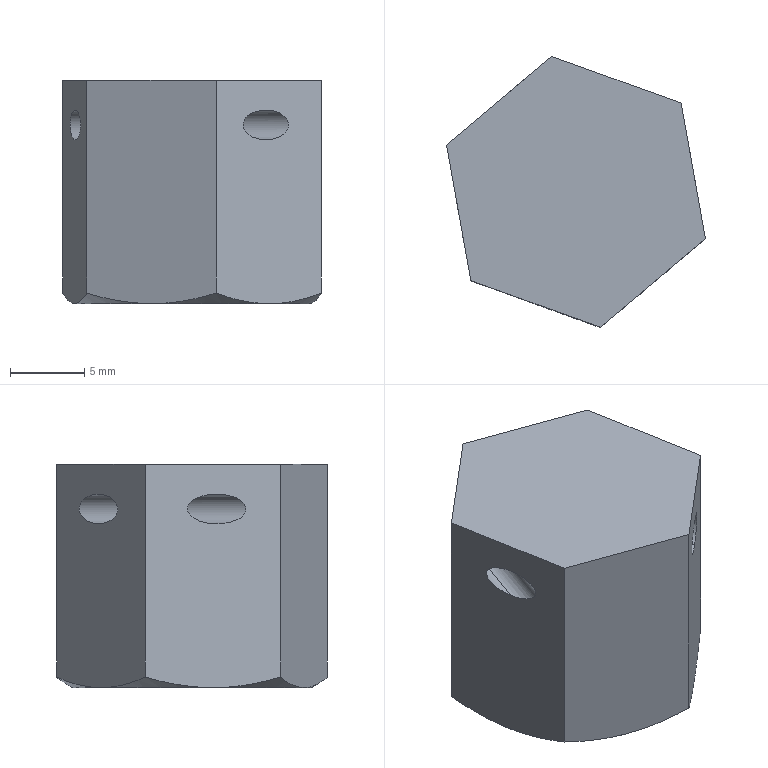Part | SolidWorks | features BaseBody 1 | 1 solid | 18 faces | box 17.375 x 18.187 x 15 mm | volume 3268 mm3 | plane 8 | cone 6 | cylinder 4 | commonest cylinder face diameters 2 x4
STEP:
#1=CARTESIAN_POINT('',(-39.503,-11.386,-260.55));
#2=VERTEX_POINT('',#1);
#3=CARTESIAN_POINT('',(-39.503,-11.386,-258.55));
#4=VERTEX_POINT('',#3);
#5=CARTESIAN_POINT('',(-39.503,-11.386,-260.55));
#6=CARTESIAN_POINT('',(-42.561,-13.964,-260.55));
#7=CARTESIAN_POINT('',(-42.561,-13.964,-258.55));
#8=CARTESIAN_POINT('',(-39.503,-11.386,-258.55));
#9=(BOUNDED_CURVE()B_SPLINE_CURVE(3,(#5,#6,#7,#8),.UNSPECIFIED.,.F.,.F.)B_SPLINE_CURVE_WITH_KNOTS((4,4),(1.571,4.712),.UNSPECIFIED.)CURVE()GEOMETRIC_REPRESENTATION_ITEM()RATIONAL_B_SPLINE_CURVE((1.,0.3333,0.3333,1.))REPRESENTATION_ITEM(''));
#10=EDGE_CURVE('',#2,#4,#9,.T.);
#11=ORIENTED_EDGE('',*,*,#10,.F.);
#12=CARTESIAN_POINT('',(-36.633,-3.444,-260.55));
#13=VERTEX_POINT('',#12);
#14=CARTESIAN_POINT('',(-40.617,-14.469,-260.55));
#15=DIRECTION('',(0.3399,0.9405,0.));
#16=VECTOR('',#15,1000.);
#17=LINE('',#14,#16);
#18=EDGE_CURVE('',#2,#13,#17,.T.);
#19=ORIENTED_EDGE('',*,*,#18,.T.);
#20=CARTESIAN_POINT('',(-36.633,-3.444,-258.55));
#21=VERTEX_POINT('',#20);
#22=CARTESIAN_POINT('',(-36.633,-3.444,-258.55));
#23=CARTESIAN_POINT('',(-37.336,0.4933,-258.55));
#24=CARTESIAN_POINT('',(-37.336,0.4933,-260.55));
#25=CARTESIAN_POINT('',(-36.633,-3.444,-260.55));
#26=(BOUNDED_CURVE()B_SPLINE_CURVE(3,(#22,#23,#24,#25),.UNSPECIFIED.,.F.,.T.)B_SPLINE_CURVE_WITH_KNOTS((4,4),(4.712,7.854),.UNSPECIFIED.)CURVE()GEOMETRIC_REPRESENTATION_ITEM()RATIONAL_B_SPLINE_CURVE((1.,0.3333,0.3333,1.))REPRESENTATION_ITEM(''));
#27=EDGE_CURVE('',#21,#13,#26,.T.);
#28=ORIENTED_EDGE('',*,*,#27,.F.);
#29=CARTESIAN_POINT('',(-40.617,-14.469,-258.55));
#30=DIRECTION('',(0.3399,0.9405,0.));
#31=VECTOR('',#30,1000.);
#32=LINE('',#29,#31);
#33=EDGE_CURVE('',#4,#21,#32,.T.);
#34=ORIENTED_EDGE('',*,*,#33,.F.);
#35=EDGE_LOOP('',(#11,#19,#28,#34));
#36=FACE_OUTER_BOUND('',#35,.T.);
#37=CARTESIAN_POINT('',(-40.617,-14.469,-259.55));
#38=DIRECTION('',(0.3399,0.9405,0.));
#39=DIRECTION('',(0.,0.,1.));
#40=AXIS2_PLACEMENT_3D('',#37,#38,#39);
#41=CYLINDRICAL_SURFACE('',#40,1.);
#42=ADVANCED_FACE('',(#36),#41,.F.);
#43=CARTESIAN_POINT('',(-52.293,-6.763,-260.55));
#44=VERTEX_POINT('',#43);
#45=CARTESIAN_POINT('',(-52.293,-6.763,-258.55));
#46=VERTEX_POINT('',#45);
#47=CARTESIAN_POINT('',(-52.293,-6.763,-260.55));
#48=CARTESIAN_POINT('',(-52.997,-2.826,-260.55));
#49=CARTESIAN_POINT('',(-52.997,-2.826,-258.55));
#50=CARTESIAN_POINT('',(-52.293,-6.763,-258.55));
#51=(BOUNDED_CURVE()B_SPLINE_CURVE(3,(#47,#48,#49,#50),.UNSPECIFIED.,.F.,.F.)B_SPLINE_CURVE_WITH_KNOTS((4,4),(4.712,7.854),.UNSPECIFIED.)CURVE()GEOMETRIC_REPRESENTATION_ITEM()RATIONAL_B_SPLINE_CURVE((1.,0.3333,0.3333,1.))REPRESENTATION_ITEM(''));
#52=EDGE_CURVE('',#44,#46,#51,.T.);
#53=ORIENTED_EDGE('',*,*,#52,.F.);
#54=CARTESIAN_POINT('',(-49.423,1.178,-260.55));
#55=VERTEX_POINT('',#54);
#56=CARTESIAN_POINT('',(-53.407,-9.846,-260.55));
#57=DIRECTION('',(0.3399,0.9405,0.));
#58=VECTOR('',#57,1000.);
#59=LINE('',#56,#58);
#60=EDGE_CURVE('',#44,#55,#59,.T.);
#61=ORIENTED_EDGE('',*,*,#60,.T.);
#62=CARTESIAN_POINT('',(-49.423,1.178,-258.55));
#63=VERTEX_POINT('',#62);
#64=CARTESIAN_POINT('',(-49.423,1.178,-258.55));
#65=CARTESIAN_POINT('',(-52.481,-1.4,-258.55));
#66=CARTESIAN_POINT('',(-52.481,-1.4,-260.55));
#67=CARTESIAN_POINT('',(-49.423,1.178,-260.55));
#68=(BOUNDED_CURVE()B_SPLINE_CURVE(3,(#64,#65,#66,#67),.UNSPECIFIED.,.F.,.F.)B_SPLINE_CURVE_WITH_KNOTS((4,4),(1.571,4.712),.UNSPECIFIED.)CURVE()GEOMETRIC_REPRESENTATION_ITEM()RATIONAL_B_SPLINE_CURVE((1.,0.3333,0.3333,1.))REPRESENTATION_ITEM(''));
#69=EDGE_CURVE('',#63,#55,#68,.T.);
#70=ORIENTED_EDGE('',*,*,#69,.F.);
#71=CARTESIAN_POINT('',(-53.407,-9.846,-258.55));
#72=DIRECTION('',(0.3399,0.9405,0.));
#73=VECTOR('',#72,1000.);
#74=LINE('',#71,#73);
#75=EDGE_CURVE('',#46,#63,#74,.T.);
#76=ORIENTED_EDGE('',*,*,#75,.F.);
#77=EDGE_LOOP('',(#53,#61,#70,#76));
#78=FACE_OUTER_BOUND('',#77,.T.);
#79=CARTESIAN_POINT('',(-53.407,-9.846,-259.55));
#80=DIRECTION('',(0.3399,0.9405,0.));
#81=DIRECTION('',(0.,0.,1.));
#82=AXIS2_PLACEMENT_3D('',#79,#80,#81);
#83=CYLINDRICAL_SURFACE('',#82,1.);
#84=ADVANCED_FACE('',(#78),#83,.F.);
#85=ORIENTED_EDGE('',*,*,#60,.F.);
#86=CARTESIAN_POINT('',(-52.293,-6.763,-258.55));
#87=CARTESIAN_POINT('',(-51.59,-10.701,-258.55));
#88=CARTESIAN_POINT('',(-51.59,-10.701,-260.55));
#89=CARTESIAN_POINT('',(-52.293,-6.763,-260.55));
#90=(BOUNDED_CURVE()B_SPLINE_CURVE(3,(#86,#87,#88,#89),.UNSPECIFIED.,.F.,.F.)B_SPLINE_CURVE_WITH_KNOTS((4,4),(1.571,4.712),.UNSPECIFIED.)CURVE()GEOMETRIC_REPRESENTATION_ITEM()RATIONAL_B_SPLINE_CURVE((1.,0.3333,0.3333,1.))REPRESENTATION_ITEM(''));
#91=EDGE_CURVE('',#46,#44,#90,.T.);
#92=ORIENTED_EDGE('',*,*,#91,.F.);
#93=ORIENTED_EDGE('',*,*,#75,.T.);
#94=CARTESIAN_POINT('',(-49.423,1.178,-260.55));
#95=CARTESIAN_POINT('',(-46.365,3.756,-260.55));
#96=CARTESIAN_POINT('',(-46.365,3.756,-258.55));
#97=CARTESIAN_POINT('',(-49.423,1.178,-258.55));
#98=(BOUNDED_CURVE()B_SPLINE_CURVE(3,(#94,#95,#96,#97),.UNSPECIFIED.,.F.,.T.)B_SPLINE_CURVE_WITH_KNOTS((4,4),(4.712,7.854),.UNSPECIFIED.)CURVE()GEOMETRIC_REPRESENTATION_ITEM()RATIONAL_B_SPLINE_CURVE((1.,0.3333,0.3333,1.))REPRESENTATION_ITEM(''));
#99=EDGE_CURVE('',#55,#63,#98,.T.);
#100=ORIENTED_EDGE('',*,*,#99,.F.);
#101=EDGE_LOOP('',(#85,#92,#93,#100));
#102=FACE_OUTER_BOUND('',#101,.T.);
#103=CARTESIAN_POINT('',(-53.407,-9.846,-259.55));
#104=DIRECTION('',(0.3399,0.9405,0.));
#105=DIRECTION('',(0.,0.,1.));
#106=AXIS2_PLACEMENT_3D('',#103,#104,#105);
#107=CYLINDRICAL_SURFACE('',#106,1.);
#108=ADVANCED_FACE('',(#102),#107,.F.);
#109=ORIENTED_EDGE('',*,*,#18,.F.);
#110=CARTESIAN_POINT('',(-39.503,-11.386,-258.55));
#111=CARTESIAN_POINT('',(-36.444,-8.808,-258.55));
#112=CARTESIAN_POINT('',(-36.444,-8.808,-260.55));
#113=CARTESIAN_POINT('',(-39.503,-11.386,-260.55));
#114=(BOUNDED_CURVE()B_SPLINE_CURVE(3,(#110,#111,#112,#113),.UNSPECIFIED.,.F.,.F.)B_SPLINE_CURVE_WITH_KNOTS((4,4),(4.712,7.854),.UNSPECIFIED.)CURVE()GEOMETRIC_REPRESENTATION_ITEM()RATIONAL_B_SPLINE_CURVE((1.,0.3333,0.3333,1.))REPRESENTATION_ITEM(''));
#115=EDGE_CURVE('',#4,#2,#114,.T.);
#116=ORIENTED_EDGE('',*,*,#115,.F.);
#117=ORIENTED_EDGE('',*,*,#33,.T.);
#118=CARTESIAN_POINT('',(-36.633,-3.444,-260.55));
#119=CARTESIAN_POINT('',(-35.929,-7.382,-260.55));
#120=CARTESIAN_POINT('',(-35.929,-7.382,-258.55));
#121=CARTESIAN_POINT('',(-36.633,-3.444,-258.55));
#122=(BOUNDED_CURVE()B_SPLINE_CURVE(3,(#118,#119,#120,#121),.UNSPECIFIED.,.F.,.F.)B_SPLINE_CURVE_WITH_KNOTS((4,4),(1.571,4.712),.UNSPECIFIED.)CURVE()GEOMETRIC_REPRESENTATION_ITEM()RATIONAL_B_SPLINE_CURVE((1.,0.3333,0.3333,1.))REPRESENTATION_ITEM(''));
#123=EDGE_CURVE('',#13,#21,#122,.T.);
#124=ORIENTED_EDGE('',*,*,#123,.F.);
#125=EDGE_LOOP('',(#109,#116,#117,#124));
#126=FACE_OUTER_BOUND('',#125,.T.);
#127=CARTESIAN_POINT('',(-40.617,-14.469,-259.55));
#128=DIRECTION('',(0.3399,0.9405,0.));
#129=DIRECTION('',(0.,0.,1.));
#130=AXIS2_PLACEMENT_3D('',#127,#128,#129);
#131=CYLINDRICAL_SURFACE('',#130,1.);
#132=ADVANCED_FACE('',(#126),#131,.F.);
#133=CARTESIAN_POINT('',(-41.744,2.42,-271.55));
#134=VERTEX_POINT('',#133);
#135=CARTESIAN_POINT('',(-49.619,1.013,-271.55));
#136=VERTEX_POINT('',#135);
#137=CARTESIAN_POINT('',(-44.463,-5.104,-271.55));
#138=DIRECTION('',(0.,0.,1.));
#139=DIRECTION('',(0.3399,0.9405,0.));
#140=AXIS2_PLACEMENT_3D('',#137,#138,#139);
#141=CIRCLE('',#140,8.);
#142=EDGE_CURVE('',#134,#136,#141,.T.);
#143=ORIENTED_EDGE('',*,*,#142,.F.);
#144=CARTESIAN_POINT('',(-36.588,-3.697,-271.55));
#145=VERTEX_POINT('',#144);
#146=CARTESIAN_POINT('',(-44.463,-5.104,-271.55));
#147=DIRECTION('',(0.,0.,-1.));
#148=DIRECTION('',(0.3399,0.9405,0.));
#149=AXIS2_PLACEMENT_3D('',#146,#147,#148);
#150=CIRCLE('',#149,8.);
#151=EDGE_CURVE('',#134,#145,#150,.T.);
#152=ORIENTED_EDGE('',*,*,#151,.T.);
#153=CARTESIAN_POINT('',(-39.307,-11.22,-271.55));
#154=VERTEX_POINT('',#153);
#155=CARTESIAN_POINT('',(-44.463,-5.104,-271.55));
#156=DIRECTION('',(0.,0.,1.));
#157=DIRECTION('',(0.3399,0.9405,0.));
#158=AXIS2_PLACEMENT_3D('',#155,#156,#157);
#159=CIRCLE('',#158,8.);
#160=EDGE_CURVE('',#154,#145,#159,.T.);
#161=ORIENTED_EDGE('',*,*,#160,.F.);
#162=CARTESIAN_POINT('',(-47.182,-12.628,-271.55));
#163=VERTEX_POINT('',#162);
#164=CARTESIAN_POINT('',(-44.463,-5.104,-271.55));
#165=DIRECTION('',(0.,0.,1.));
#166=DIRECTION('',(0.3399,0.9405,0.));
#167=AXIS2_PLACEMENT_3D('',#164,#165,#166);
#168=CIRCLE('',#167,8.);
#169=EDGE_CURVE('',#163,#154,#168,.T.);
#170=ORIENTED_EDGE('',*,*,#169,.F.);
#171=CARTESIAN_POINT('',(-52.338,-6.511,-271.55));
#172=VERTEX_POINT('',#171);
#173=CARTESIAN_POINT('',(-44.463,-5.104,-271.55));
#174=DIRECTION('',(0.,0.,1.));
#175=DIRECTION('',(0.3399,0.9405,0.));
#176=AXIS2_PLACEMENT_3D('',#173,#174,#175);
#177=CIRCLE('',#176,8.);
#178=EDGE_CURVE('',#172,#163,#177,.T.);
#179=ORIENTED_EDGE('',*,*,#178,.F.);
#180=CARTESIAN_POINT('',(-44.463,-5.104,-271.55));
#181=DIRECTION('',(0.,0.,1.));
#182=DIRECTION('',(0.3399,0.9405,0.));
#183=AXIS2_PLACEMENT_3D('',#180,#181,#182);
#184=CIRCLE('',#183,8.);
#185=EDGE_CURVE('',#136,#172,#184,.T.);
#186=ORIENTED_EDGE('',*,*,#185,.F.);
#187=EDGE_LOOP('',(#143,#152,#161,#170,#179,#186));
#188=FACE_OUTER_BOUND('',#187,.T.);
#189=CARTESIAN_POINT('',(-34.15,-17.337,-271.55));
#190=DIRECTION('',(0.,0.,-1.));
#191=DIRECTION('',(0.,-1.,0.));
#192=AXIS2_PLACEMENT_3D('',#189,#190,#191);
#193=PLANE('',#192);
#194=ADVANCED_FACE('',(#188),#193,.T.);
#195=CARTESIAN_POINT('',(-46.088,3.99,-270.835));
#196=VERTEX_POINT('',#195);
#197=CARTESIAN_POINT('',(-41.744,2.42,-271.55));
#198=CARTESIAN_POINT('',(-42.485,2.688,-271.55));
#199=CARTESIAN_POINT('',(-43.216,2.952,-271.482));
#200=CARTESIAN_POINT('',(-44.663,3.475,-271.233));
#201=CARTESIAN_POINT('',(-45.378,3.733,-271.053));
#202=CARTESIAN_POINT('',(-46.088,3.99,-270.835));
#203=B_SPLINE_CURVE_WITH_KNOTS('',3,(#197,#198,#199,#200,#201,#202),.UNSPECIFIED.,.F.,.F.,(4,2,4),(0.,0.002337,0.004674),.UNSPECIFIED.);
#204=EDGE_CURVE('',#134,#196,#203,.T.);
#205=ORIENTED_EDGE('',*,*,#204,.F.);
#206=ORIENTED_EDGE('',*,*,#142,.T.);
#207=CARTESIAN_POINT('',(-46.088,3.99,-270.835));
#208=CARTESIAN_POINT('',(-46.665,3.504,-271.053));
#209=CARTESIAN_POINT('',(-47.246,3.013,-271.233));
#210=CARTESIAN_POINT('',(-48.422,2.022,-271.482));
#211=CARTESIAN_POINT('',(-49.016,1.521,-271.55));
#212=CARTESIAN_POINT('',(-49.619,1.013,-271.55));
#213=B_SPLINE_CURVE_WITH_KNOTS('',3,(#207,#208,#209,#210,#211,#212),.UNSPECIFIED.,.F.,.F.,(4,2,4),(0.,0.002337,0.004674),.UNSPECIFIED.);
#214=EDGE_CURVE('',#196,#136,#213,.T.);
#215=ORIENTED_EDGE('',*,*,#214,.F.);
#216=EDGE_LOOP('',(#205,#206,#215));
#217=FACE_OUTER_BOUND('',#216,.T.);
#218=CARTESIAN_POINT('',(-44.463,-5.104,-267.662));
#219=DIRECTION('',(0.,0.,1.));
#220=DIRECTION('',(-0.3399,-0.9405,0.));
#221=AXIS2_PLACEMENT_3D('',#218,#219,#220);
#222=CONICAL_SURFACE('',#221,14.733,1.047);
#223=ADVANCED_FACE('',(#217),#222,.T.);
#224=CARTESIAN_POINT('',(-53.151,-1.964,-270.835));
#225=VERTEX_POINT('',#224);
#226=CARTESIAN_POINT('',(-49.619,1.013,-271.55));
#227=CARTESIAN_POINT('',(-50.222,0.5049,-271.55));
#228=CARTESIAN_POINT('',(-50.816,0.003642,-271.482));
#229=CARTESIAN_POINT('',(-51.992,-0.9876,-271.233));
#230=CARTESIAN_POINT('',(-52.574,-1.478,-271.053));
#231=CARTESIAN_POINT('',(-53.151,-1.964,-270.835));
#232=B_SPLINE_CURVE_WITH_KNOTS('',3,(#226,#227,#228,#229,#230,#231),.UNSPECIFIED.,.F.,.F.,(4,2,4),(0.,0.002337,0.004674),.UNSPECIFIED.);
#233=EDGE_CURVE('',#136,#225,#232,.T.);
#234=ORIENTED_EDGE('',*,*,#233,.F.);
#235=ORIENTED_EDGE('',*,*,#185,.T.);
#236=CARTESIAN_POINT('',(-53.151,-1.964,-270.835));
#237=CARTESIAN_POINT('',(-53.018,-2.707,-271.053));
#238=CARTESIAN_POINT('',(-52.884,-3.455,-271.233));
#239=CARTESIAN_POINT('',(-52.614,-4.969,-271.482));
#240=CARTESIAN_POINT('',(-52.477,-5.735,-271.55));
#241=CARTESIAN_POINT('',(-52.338,-6.511,-271.55));
#242=B_SPLINE_CURVE_WITH_KNOTS('',3,(#236,#237,#238,#239,#240,#241),.UNSPECIFIED.,.F.,.F.,(4,2,4),(0.,0.002337,0.004674),.UNSPECIFIED.);
#243=EDGE_CURVE('',#225,#172,#242,.T.);
#244=ORIENTED_EDGE('',*,*,#243,.F.);
#245=EDGE_LOOP('',(#234,#235,#244));
#246=FACE_OUTER_BOUND('',#245,.T.);
#247=CARTESIAN_POINT('',(-44.463,-5.104,-267.662));
#248=DIRECTION('',(0.,0.,1.));
#249=DIRECTION('',(-0.3399,-0.9405,0.));
#250=AXIS2_PLACEMENT_3D('',#247,#248,#249);
#251=CONICAL_SURFACE('',#250,14.733,1.047);
#252=ADVANCED_FACE('',(#246),#251,.T.);
#253=CARTESIAN_POINT('',(-51.526,-11.058,-270.835));
#254=VERTEX_POINT('',#253);
#255=CARTESIAN_POINT('',(-52.338,-6.511,-271.55));
#256=CARTESIAN_POINT('',(-52.2,-7.287,-271.55));
#257=CARTESIAN_POINT('',(-52.063,-8.052,-271.482));
#258=CARTESIAN_POINT('',(-51.792,-9.566,-271.233));
#259=CARTESIAN_POINT('',(-51.659,-10.315,-271.053));
#260=CARTESIAN_POINT('',(-51.526,-11.058,-270.835));
#261=B_SPLINE_CURVE_WITH_KNOTS('',3,(#255,#256,#257,#258,#259,#260),.UNSPECIFIED.,.F.,.F.,(4,2,4),(0.,0.002337,0.004674),.UNSPECIFIED.);
#262=EDGE_CURVE('',#172,#254,#261,.T.);
#263=ORIENTED_EDGE('',*,*,#262,.F.);
#264=ORIENTED_EDGE('',*,*,#178,.T.);
#265=CARTESIAN_POINT('',(-51.526,-11.058,-270.835));
#266=CARTESIAN_POINT('',(-50.816,-11.314,-271.053));
#267=CARTESIAN_POINT('',(-50.101,-11.573,-271.233));
#268=CARTESIAN_POINT('',(-48.655,-12.095,-271.482));
#269=CARTESIAN_POINT('',(-47.923,-12.36,-271.55));
#270=CARTESIAN_POINT('',(-47.182,-12.628,-271.55));
#271=B_SPLINE_CURVE_WITH_KNOTS('',3,(#265,#266,#267,#268,#269,#270),.UNSPECIFIED.,.F.,.F.,(4,2,4),(0.,0.002337,0.004674),.UNSPECIFIED.);
#272=EDGE_CURVE('',#254,#163,#271,.T.);
#273=ORIENTED_EDGE('',*,*,#272,.F.);
#274=EDGE_LOOP('',(#263,#264,#273));
#275=FACE_OUTER_BOUND('',#274,.T.);
#276=CARTESIAN_POINT('',(-44.463,-5.104,-267.662));
#277=DIRECTION('',(0.,0.,1.));
#278=DIRECTION('',(-0.3399,-0.9405,0.));
#279=AXIS2_PLACEMENT_3D('',#276,#277,#278);
#280=CONICAL_SURFACE('',#279,14.733,1.047);
#281=ADVANCED_FACE('',(#275),#280,.T.);
#282=ORIENTED_EDGE('',*,*,#169,.T.);
#283=CARTESIAN_POINT('',(-42.838,-14.197,-270.835));
#284=VERTEX_POINT('',#283);
#285=CARTESIAN_POINT('',(-42.838,-14.197,-270.835));
#286=CARTESIAN_POINT('',(-42.261,-13.711,-271.053));
#287=CARTESIAN_POINT('',(-41.68,-13.221,-271.233));
#288=CARTESIAN_POINT('',(-40.504,-12.23,-271.482));
#289=CARTESIAN_POINT('',(-39.909,-11.728,-271.55));
#290=CARTESIAN_POINT('',(-39.307,-11.22,-271.55));
#291=B_SPLINE_CURVE_WITH_KNOTS('',3,(#285,#286,#287,#288,#289,#290),.UNSPECIFIED.,.F.,.F.,(4,2,4),(0.,0.002337,0.004674),.UNSPECIFIED.);
#292=EDGE_CURVE('',#284,#154,#291,.T.);
#293=ORIENTED_EDGE('',*,*,#292,.F.);
#294=CARTESIAN_POINT('',(-47.182,-12.628,-271.55));
#295=CARTESIAN_POINT('',(-46.441,-12.895,-271.55));
#296=CARTESIAN_POINT('',(-45.709,-13.16,-271.482));
#297=CARTESIAN_POINT('',(-44.263,-13.682,-271.233));
#298=CARTESIAN_POINT('',(-43.548,-13.941,-271.053));
#299=CARTESIAN_POINT('',(-42.838,-14.197,-270.835));
#300=B_SPLINE_CURVE_WITH_KNOTS('',3,(#294,#295,#296,#297,#298,#299),.UNSPECIFIED.,.F.,.F.,(4,2,4),(0.,0.002337,0.004674),.UNSPECIFIED.);
#301=EDGE_CURVE('',#163,#284,#300,.T.);
#302=ORIENTED_EDGE('',*,*,#301,.F.);
#303=EDGE_LOOP('',(#282,#293,#302));
#304=FACE_OUTER_BOUND('',#303,.T.);
#305=CARTESIAN_POINT('',(-44.463,-5.104,-267.662));
#306=DIRECTION('',(0.,0.,1.));
#307=DIRECTION('',(-0.3399,-0.9405,0.));
#308=AXIS2_PLACEMENT_3D('',#305,#306,#307);
#309=CONICAL_SURFACE('',#308,14.733,1.047);
#310=ADVANCED_FACE('',(#304),#309,.T.);
#311=ORIENTED_EDGE('',*,*,#160,.T.);
#312=CARTESIAN_POINT('',(-35.775,-8.244,-270.835));
#313=VERTEX_POINT('',#312);
#314=CARTESIAN_POINT('',(-35.775,-8.244,-270.835));
#315=CARTESIAN_POINT('',(-35.908,-7.501,-271.053));
#316=CARTESIAN_POINT('',(-36.042,-6.752,-271.233));
#317=CARTESIAN_POINT('',(-36.312,-5.238,-271.482));
#318=CARTESIAN_POINT('',(-36.449,-4.473,-271.55));
#319=CARTESIAN_POINT('',(-36.588,-3.697,-271.55));
#320=B_SPLINE_CURVE_WITH_KNOTS('',3,(#314,#315,#316,#317,#318,#319),.UNSPECIFIED.,.F.,.F.,(4,2,4),(0.,0.002337,0.004674),.UNSPECIFIED.);
#321=EDGE_CURVE('',#313,#145,#320,.T.);
#322=ORIENTED_EDGE('',*,*,#321,.F.);
#323=CARTESIAN_POINT('',(-39.307,-11.22,-271.55));
#324=CARTESIAN_POINT('',(-38.704,-10.712,-271.55));
#325=CARTESIAN_POINT('',(-38.109,-10.211,-271.482));
#326=CARTESIAN_POINT('',(-36.934,-9.22,-271.233));
#327=CARTESIAN_POINT('',(-36.352,-8.73,-271.053));
#328=CARTESIAN_POINT('',(-35.775,-8.244,-270.835));
#329=B_SPLINE_CURVE_WITH_KNOTS('',3,(#323,#324,#325,#326,#327,#328),.UNSPECIFIED.,.F.,.F.,(4,2,4),(0.,0.002337,0.004674),.UNSPECIFIED.);
#330=EDGE_CURVE('',#154,#313,#329,.T.);
#331=ORIENTED_EDGE('',*,*,#330,.F.);
#332=EDGE_LOOP('',(#311,#322,#331));
#333=FACE_OUTER_BOUND('',#332,.T.);
#334=CARTESIAN_POINT('',(-44.463,-5.104,-267.662));
#335=DIRECTION('',(0.,0.,1.));
#336=DIRECTION('',(-0.3399,-0.9405,0.));
#337=AXIS2_PLACEMENT_3D('',#334,#335,#336);
#338=CONICAL_SURFACE('',#337,14.733,1.047);
#339=ADVANCED_FACE('',(#333),#338,.T.);
#340=ORIENTED_EDGE('',*,*,#151,.F.);
#341=CARTESIAN_POINT('',(-37.4,0.8501,-270.835));
#342=VERTEX_POINT('',#341);
#343=CARTESIAN_POINT('',(-37.4,0.8501,-270.835));
#344=CARTESIAN_POINT('',(-38.11,1.107,-271.053));
#345=CARTESIAN_POINT('',(-38.825,1.365,-271.233));
#346=CARTESIAN_POINT('',(-40.271,1.888,-271.482));
#347=CARTESIAN_POINT('',(-41.002,2.152,-271.55));
#348=CARTESIAN_POINT('',(-41.744,2.42,-271.55));
#349=B_SPLINE_CURVE_WITH_KNOTS('',3,(#343,#344,#345,#346,#347,#348),.UNSPECIFIED.,.F.,.F.,(4,2,4),(0.,0.002337,0.004674),.UNSPECIFIED.);
#350=EDGE_CURVE('',#342,#134,#349,.T.);
#351=ORIENTED_EDGE('',*,*,#350,.F.);
#352=CARTESIAN_POINT('',(-36.588,-3.697,-271.55));
#353=CARTESIAN_POINT('',(-36.726,-2.921,-271.55));
#354=CARTESIAN_POINT('',(-36.863,-2.155,-271.482));
#355=CARTESIAN_POINT('',(-37.133,-0.6413,-271.233));
#356=CARTESIAN_POINT('',(-37.267,0.1073,-271.053));
#357=CARTESIAN_POINT('',(-37.4,0.8501,-270.835));
#358=B_SPLINE_CURVE_WITH_KNOTS('',3,(#352,#353,#354,#355,#356,#357),.UNSPECIFIED.,.F.,.F.,(4,2,4),(0.,0.002337,0.004674),.UNSPECIFIED.);
#359=EDGE_CURVE('',#145,#342,#358,.T.);
#360=ORIENTED_EDGE('',*,*,#359,.F.);
#361=EDGE_LOOP('',(#340,#351,#360));
#362=FACE_OUTER_BOUND('',#361,.T.);
#363=CARTESIAN_POINT('',(-44.463,-5.104,-267.662));
#364=DIRECTION('',(0.,0.,1.));
#365=DIRECTION('',(-0.3399,-0.9405,0.));
#366=AXIS2_PLACEMENT_3D('',#363,#364,#365);
#367=CONICAL_SURFACE('',#366,14.733,1.047);
#368=ADVANCED_FACE('',(#362),#367,.T.);
#369=CARTESIAN_POINT('',(-37.4,0.8501,-256.55));
#370=VERTEX_POINT('',#369);
#371=CARTESIAN_POINT('',(-35.775,-8.244,-256.55));
#372=VERTEX_POINT('',#371);
#373=CARTESIAN_POINT('',(-37.4,0.8501,-256.55));
#374=DIRECTION('',(0.1759,-0.9844,0.));
#375=VECTOR('',#374,1000.);
#376=LINE('',#373,#375);
#377=EDGE_CURVE('',#370,#372,#376,.T.);
#378=ORIENTED_EDGE('',*,*,#377,.F.);
#379=CARTESIAN_POINT('',(-46.088,3.99,-256.55));
#380=VERTEX_POINT('',#379);
#381=CARTESIAN_POINT('',(-46.088,3.99,-256.55));
#382=DIRECTION('',(0.9405,-0.3399,0.));
#383=VECTOR('',#382,1000.);
#384=LINE('',#381,#383);
#385=EDGE_CURVE('',#380,#370,#384,.T.);
#386=ORIENTED_EDGE('',*,*,#385,.F.);
#387=CARTESIAN_POINT('',(-53.151,-1.964,-256.55));
#388=VERTEX_POINT('',#387);
#389=CARTESIAN_POINT('',(-53.151,-1.964,-256.55));
#390=DIRECTION('',(0.7646,0.6445,0.));
#391=VECTOR('',#390,1000.);
#392=LINE('',#389,#391);
#393=EDGE_CURVE('',#388,#380,#392,.T.);
#394=ORIENTED_EDGE('',*,*,#393,.F.);
#395=CARTESIAN_POINT('',(-51.526,-11.058,-256.55));
#396=VERTEX_POINT('',#395);
#397=CARTESIAN_POINT('',(-51.526,-11.058,-256.55));
#398=DIRECTION('',(-0.1759,0.9844,0.));
#399=VECTOR('',#398,1000.);
#400=LINE('',#397,#399);
#401=EDGE_CURVE('',#396,#388,#400,.T.);
#402=ORIENTED_EDGE('',*,*,#401,.F.);
#403=CARTESIAN_POINT('',(-42.838,-14.197,-256.55));
#404=VERTEX_POINT('',#403);
#405=CARTESIAN_POINT('',(-42.838,-14.197,-256.55));
#406=DIRECTION('',(-0.9405,0.3399,0.));
#407=VECTOR('',#406,1000.);
#408=LINE('',#405,#407);
#409=EDGE_CURVE('',#404,#396,#408,.T.);
#410=ORIENTED_EDGE('',*,*,#409,.F.);
#411=CARTESIAN_POINT('',(-35.775,-8.244,-256.55));
#412=DIRECTION('',(-0.7646,-0.6445,0.));
#413=VECTOR('',#412,1000.);
#414=LINE('',#411,#413);
#415=EDGE_CURVE('',#372,#404,#414,.T.);
#416=ORIENTED_EDGE('',*,*,#415,.F.);
#417=EDGE_LOOP('',(#378,#386,#394,#402,#410,#416));
#418=FACE_OUTER_BOUND('',#417,.T.);
#419=CARTESIAN_POINT('',(-34.15,-17.337,-256.55));
#420=DIRECTION('',(0.,0.,-1.));
#421=DIRECTION('',(0.,-1.,0.));
#422=AXIS2_PLACEMENT_3D('',#419,#420,#421);
#423=PLANE('',#422);
#424=ADVANCED_FACE('',(#418),#423,.F.);
#425=CARTESIAN_POINT('',(-37.4,0.8501,-271.55));
#426=DIRECTION('',(0.,0.,1.));
#427=VECTOR('',#426,1000.);
#428=LINE('',#425,#427);
#429=EDGE_CURVE('',#342,#370,#428,.T.);
#430=ORIENTED_EDGE('',*,*,#429,.F.);
#431=ORIENTED_EDGE('',*,*,#350,.T.);
#432=ORIENTED_EDGE('',*,*,#204,.T.);
#433=CARTESIAN_POINT('',(-46.088,3.99,-271.55));
#434=DIRECTION('',(0.,0.,1.));
#435=VECTOR('',#434,1000.);
#436=LINE('',#433,#435);
#437=EDGE_CURVE('',#196,#380,#436,.T.);
#438=ORIENTED_EDGE('',*,*,#437,.T.);
#439=ORIENTED_EDGE('',*,*,#385,.T.);
#440=EDGE_LOOP('',(#430,#431,#432,#438,#439));
#441=FACE_OUTER_BOUND('',#440,.T.);
#442=CARTESIAN_POINT('',(-46.088,3.99,-271.55));
#443=DIRECTION('',(-0.3399,-0.9405,0.));
#444=DIRECTION('',(-0.9405,0.3399,0.));
#445=AXIS2_PLACEMENT_3D('',#442,#443,#444);
#446=PLANE('',#445);
#447=ADVANCED_FACE('',(#441),#446,.F.);
#448=ORIENTED_EDGE('',*,*,#437,.F.);
#449=ORIENTED_EDGE('',*,*,#214,.T.);
#450=ORIENTED_EDGE('',*,*,#233,.T.);
#451=CARTESIAN_POINT('',(-53.151,-1.964,-271.55));
#452=DIRECTION('',(0.,0.,1.));
#453=VECTOR('',#452,1000.);
#454=LINE('',#451,#453);
#455=EDGE_CURVE('',#225,#388,#454,.T.);
#456=ORIENTED_EDGE('',*,*,#455,.T.);
#457=ORIENTED_EDGE('',*,*,#393,.T.);
#458=EDGE_LOOP('',(#448,#449,#450,#456,#457));
#459=FACE_OUTER_BOUND('',#458,.T.);
#460=ORIENTED_EDGE('',*,*,#69,.T.);
#461=ORIENTED_EDGE('',*,*,#99,.T.);
#462=EDGE_LOOP('',(#460,#461));
#463=FACE_BOUND('',#462,.T.);
#464=CARTESIAN_POINT('',(-53.151,-1.964,-271.55));
#465=DIRECTION('',(0.6445,-0.7646,0.));
#466=DIRECTION('',(0.,0.,-1.));
#467=AXIS2_PLACEMENT_3D('',#464,#465,#466);
#468=PLANE('',#467);
#469=ADVANCED_FACE('',(#459,#463),#468,.F.);
#470=ORIENTED_EDGE('',*,*,#455,.F.);
#471=ORIENTED_EDGE('',*,*,#243,.T.);
#472=ORIENTED_EDGE('',*,*,#262,.T.);
#473=CARTESIAN_POINT('',(-51.526,-11.058,-271.55));
#474=DIRECTION('',(0.,0.,1.));
#475=VECTOR('',#474,1000.);
#476=LINE('',#473,#475);
#477=EDGE_CURVE('',#254,#396,#476,.T.);
#478=ORIENTED_EDGE('',*,*,#477,.T.);
#479=ORIENTED_EDGE('',*,*,#401,.T.);
#480=EDGE_LOOP('',(#470,#471,#472,#478,#479));
#481=FACE_OUTER_BOUND('',#480,.T.);
#482=ORIENTED_EDGE('',*,*,#91,.T.);
#483=ORIENTED_EDGE('',*,*,#52,.T.);
#484=EDGE_LOOP('',(#482,#483));
#485=FACE_BOUND('',#484,.T.);
#486=CARTESIAN_POINT('',(-51.526,-11.058,-271.55));
#487=DIRECTION('',(0.9844,0.1759,0.));
#488=DIRECTION('',(0.,0.,-1.));
#489=AXIS2_PLACEMENT_3D('',#486,#487,#488);
#490=PLANE('',#489);
#491=ADVANCED_FACE('',(#481,#485),#490,.F.);
#492=ORIENTED_EDGE('',*,*,#477,.F.);
#493=ORIENTED_EDGE('',*,*,#272,.T.);
#494=ORIENTED_EDGE('',*,*,#301,.T.);
#495=CARTESIAN_POINT('',(-42.838,-14.197,-271.55));
#496=DIRECTION('',(0.,0.,1.));
#497=VECTOR('',#496,1000.);
#498=LINE('',#495,#497);
#499=EDGE_CURVE('',#284,#404,#498,.T.);
#500=ORIENTED_EDGE('',*,*,#499,.T.);
#501=ORIENTED_EDGE('',*,*,#409,.T.);
#502=EDGE_LOOP('',(#492,#493,#494,#500,#501));
#503=FACE_OUTER_BOUND('',#502,.T.);
#504=CARTESIAN_POINT('',(-42.838,-14.197,-271.55));
#505=DIRECTION('',(0.3399,0.9405,0.));
#506=DIRECTION('',(0.,0.,-1.));
#507=AXIS2_PLACEMENT_3D('',#504,#505,#506);
#508=PLANE('',#507);
#509=ADVANCED_FACE('',(#503),#508,.F.);
#510=ORIENTED_EDGE('',*,*,#499,.F.);
#511=ORIENTED_EDGE('',*,*,#292,.T.);
#512=ORIENTED_EDGE('',*,*,#330,.T.);
#513=CARTESIAN_POINT('',(-35.775,-8.244,-271.55));
#514=DIRECTION('',(0.,0.,1.));
#515=VECTOR('',#514,1000.);
#516=LINE('',#513,#515);
#517=EDGE_CURVE('',#313,#372,#516,.T.);
#518=ORIENTED_EDGE('',*,*,#517,.T.);
#519=ORIENTED_EDGE('',*,*,#415,.T.);
#520=EDGE_LOOP('',(#510,#511,#512,#518,#519));
#521=FACE_OUTER_BOUND('',#520,.T.);
#522=ORIENTED_EDGE('',*,*,#115,.T.);
#523=ORIENTED_EDGE('',*,*,#10,.T.);
#524=EDGE_LOOP('',(#522,#523));
#525=FACE_BOUND('',#524,.T.);
#526=CARTESIAN_POINT('',(-35.775,-8.244,-271.55));
#527=DIRECTION('',(-0.6445,0.7646,0.));
#528=DIRECTION('',(0.,0.,1.));
#529=AXIS2_PLACEMENT_3D('',#526,#527,#528);
#530=PLANE('',#529);
#531=ADVANCED_FACE('',(#521,#525),#530,.F.);
#532=ORIENTED_EDGE('',*,*,#517,.F.);
#533=ORIENTED_EDGE('',*,*,#321,.T.);
#534=ORIENTED_EDGE('',*,*,#359,.T.);
#535=ORIENTED_EDGE('',*,*,#429,.T.);
#536=ORIENTED_EDGE('',*,*,#377,.T.);
#537=EDGE_LOOP('',(#532,#533,#534,#535,#536));
#538=FACE_OUTER_BOUND('',#537,.T.);
#539=ORIENTED_EDGE('',*,*,#27,.T.);
#540=ORIENTED_EDGE('',*,*,#123,.T.);
#541=EDGE_LOOP('',(#539,#540));
#542=FACE_BOUND('',#541,.T.);
#543=CARTESIAN_POINT('',(-37.4,0.8501,-271.55));
#544=DIRECTION('',(-0.9844,-0.1759,0.));
#545=DIRECTION('',(-0.1759,0.9844,0.));
#546=AXIS2_PLACEMENT_3D('',#543,#544,#545);
#547=PLANE('',#546);
#548=ADVANCED_FACE('',(#538,#542),#547,.F.);
#549=CLOSED_SHELL('',(#42,#84,#108,#132,#194,#223,#252,#281,#310,#339,#368,#424,#447,#469,#491,#509,#531,#548));
#550=MANIFOLD_SOLID_BREP('',#549);
#551=CARTESIAN_POINT('',(0.,0.,0.));
#552=DIRECTION('',(0.,0.,1.));
#553=DIRECTION('',(1.,0.,0.));
#554=AXIS2_PLACEMENT_3D('',#551,#552,#553);
#555=(LENGTH_UNIT()NAMED_UNIT(*)SI_UNIT(.MILLI.,.METRE.));
#556=UNCERTAINTY_MEASURE_WITH_UNIT(LENGTH_MEASURE(0.00001),#555,'','');
#557=(NAMED_UNIT(*)PLANE_ANGLE_UNIT()SI_UNIT($,.RADIAN.));
#558=(NAMED_UNIT(*)SI_UNIT($,.STERADIAN.)SOLID_ANGLE_UNIT());
#559=(GEOMETRIC_REPRESENTATION_CONTEXT(3)GLOBAL_UNCERTAINTY_ASSIGNED_CONTEXT((#556))GLOBAL_UNIT_ASSIGNED_CONTEXT((#555,#557,#558))REPRESENTATION_CONTEXT('',''));
#560=ADVANCED_BREP_SHAPE_REPRESENTATION('',(#550,#554),#559);